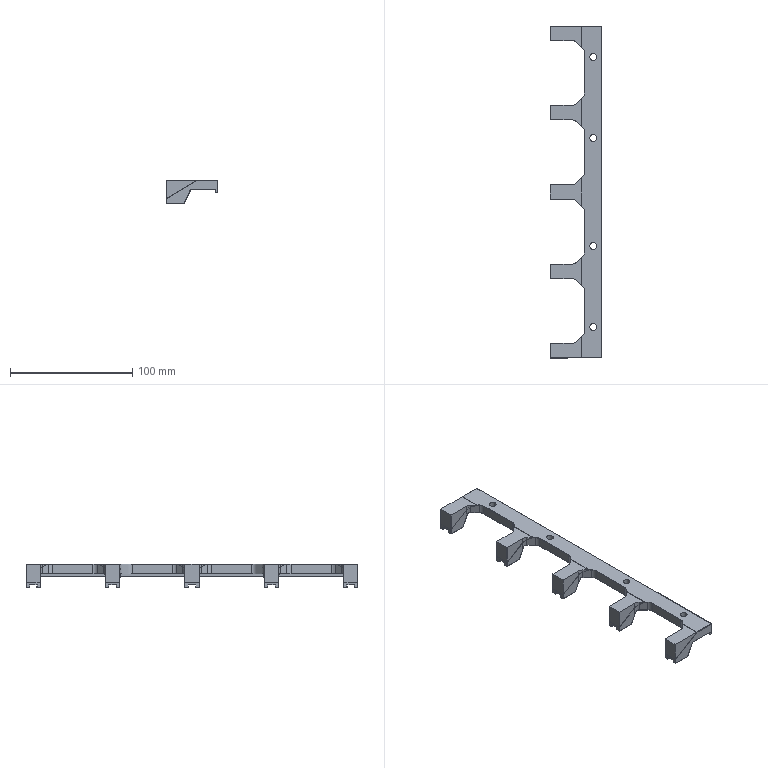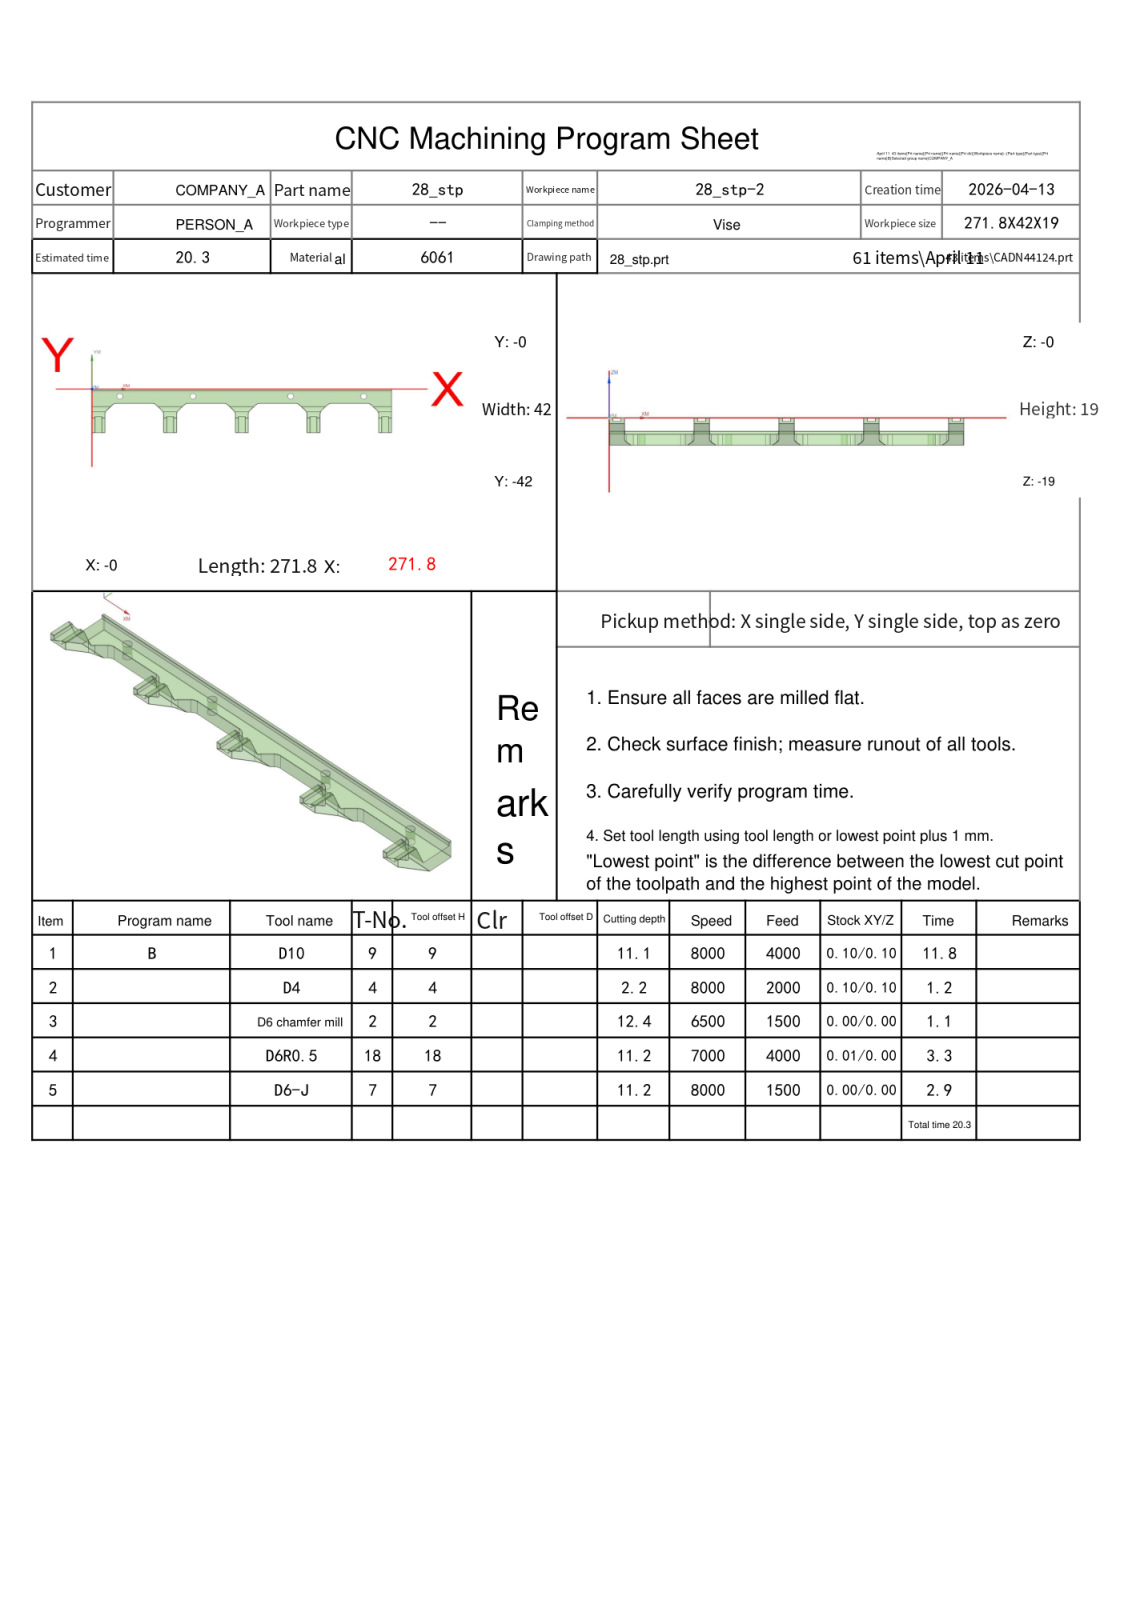NC program | NX | posted by the shop | part box 42 x 271.8 x 19 mm
Lines 6499 to 7627 of 14465:
N2 T04 M06
(D4  D=4. R=0. H=04 ce=0.10 di=0.10)
G00 G90 G54 X5.9 Y-47. M03 S8000
G43 H04 Z15.8
M08
Z1.225
G01 Z-.275 F2000.
Y-43.96
X3.71
X5. Y-42.67
Y-25.946
X3.72 Y-24.515
X8.08
X6.8 Y-25.946
Y-42.67
X8.09 Y-43.96
X5.9
X5.4
Y-47.
Z1.225
G00 X5.9
Z.95
G01 Z-.55
Y-43.96
X3.71
X5. Y-42.67
Y-25.946
X3.72 Y-24.515
X8.08
X6.8 Y-25.946
Y-42.67
X8.09 Y-43.96
X5.9
X5.4
Y-47.
Z.95
G00 X5.9
Z.675
G01 Z-.825
Y-43.96
X3.71
X5. Y-42.67
Y-25.946
X3.72 Y-24.515
X8.08
X6.8 Y-25.946
Y-42.67
X8.09 Y-43.96
X5.9
X5.4
Y-47.
Z.675
G00 X5.9
Z.4
G01 Z-1.1
Y-43.96
X3.71
X5. Y-42.67
Y-25.946
X3.72 Y-24.515
X8.08
X6.8 Y-25.946
Y-42.67
X8.09 Y-43.96
X5.9
X5.4
Y-47.
Z.4
G00 X5.9
Z.125
G01 Z-1.375
Y-43.96
X3.71
X5. Y-42.67
Y-25.946
X3.72 Y-24.515
X8.08
X6.8 Y-25.946
Y-42.67
X8.09 Y-43.96
X5.9
X5.4
Y-47.
Z.125
G00 X5.9
Z-.15
G01 Z-1.65
Y-43.96
X3.71
X5. Y-42.67
Y-25.946
X3.72 Y-24.515
X8.08
X6.8 Y-25.946
Y-42.67
X8.09 Y-43.96
X5.9
X5.4
Y-47.
Z-.15
G00 X5.9
Z-.425
G01 Z-1.925
Y-43.96
X3.71
X5. Y-42.67
Y-25.946
X3.72 Y-24.515
X8.08
X6.8 Y-25.946
Y-42.67
X8.09 Y-43.96
X5.9
X5.4
Y-47.
Z-.425
G00 X5.9
Z-.7
G01 Z-2.2
Y-43.96
X3.71
X5. Y-42.67
Y-25.946
X3.72 Y-24.515
X8.08
X6.8 Y-25.946
Y-42.67
X8.09 Y-43.96
X5.9
X5.4
Y-47.
Z-.7
G00 Z3.
X70.9
Z1.225
G01 Z-.275
Y-43.96
X68.71
X70. Y-42.67
Y-25.946
X68.72 Y-24.515
X73.08
X71.8 Y-25.946
Y-42.67
X73.09 Y-43.96
X70.9
X70.4
Y-47.
Z1.225
G00 X70.9
Z.95
G01 Z-.55
Y-43.96
X68.71
X70. Y-42.67
Y-25.946
X68.72 Y-24.515
X73.08
X71.8 Y-25.946
Y-42.67
X73.09 Y-43.96
X70.9
X70.4
Y-47.
Z.95
G00 X70.9
Z.675
G01 Z-.825
Y-43.96
X68.71
X70. Y-42.67
Y-25.946
X68.72 Y-24.515
X73.08
X71.8 Y-25.946
Y-42.67
X73.09 Y-43.96
X70.9
X70.4
Y-47.
Z.675
G00 X70.9
Z.4
G01 Z-1.1
Y-43.96
X68.71
X70. Y-42.67
Y-25.946
X68.72 Y-24.515
X73.08
X71.8 Y-25.946
Y-42.67
X73.09 Y-43.96
X70.9
X70.4
Y-47.
Z.4
G00 X70.9
Z.125
G01 Z-1.375
Y-43.96
X68.71
X70. Y-42.67
Y-25.946
X68.72 Y-24.515
X73.08
X71.8 Y-25.946
Y-42.67
X73.09 Y-43.96
X70.9
X70.4
Y-47.
Z.125
G00 X70.9
Z-.15
G01 Z-1.65
Y-43.96
X68.71
X70. Y-42.67
Y-25.946
X68.72 Y-24.515
X73.08
X71.8 Y-25.946
Y-42.67
X73.09 Y-43.96
X70.9
X70.4
Y-47.
Z-.15
G00 X70.9
Z-.425
G01 Z-1.925
Y-43.96
X68.71
X70. Y-42.67
Y-25.946
X68.72 Y-24.515
X73.08
X71.8 Y-25.946
Y-42.67
X73.09 Y-43.96
X70.9
X70.4
Y-47.
Z-.425
G00 X70.9
Z-.7
G01 Z-2.2
Y-43.96
X68.71
X70. Y-42.67
Y-25.946
X68.72 Y-24.515
X73.08
X71.8 Y-25.946
Y-42.67
X73.09 Y-43.96
X70.9
X70.4
Y-47.
Z-.7
G00 Z3.
X135.9
Z1.225
G01 Z-.275
Y-43.96
X133.71
X135. Y-42.67
Y-25.946
X133.72 Y-24.515
X138.08
X136.8 Y-25.946
Y-42.67
X138.09 Y-43.96
X135.9
X135.4
Y-47.
Z1.225
G00 X135.9
Z.95
G01 Z-.55
Y-43.96
X133.71
X135. Y-42.67
Y-25.946
X133.72 Y-24.515
X138.08
X136.8 Y-25.946
Y-42.67
X138.09 Y-43.96
X135.9
X135.4
Y-47.
Z.95
G00 X135.9
Z.675
G01 Z-.825
Y-43.96
X133.71
X135. Y-42.67
Y-25.946
X133.72 Y-24.515
X138.08
X136.8 Y-25.946
Y-42.67
X138.09 Y-43.96
X135.9
X135.4
Y-47.
Z.675
G00 X135.9
Z.4
G01 Z-1.1
Y-43.96
X133.71
X135. Y-42.67
Y-25.946
X133.72 Y-24.515
X138.08
X136.8 Y-25.946
Y-42.67
X138.09 Y-43.96
X135.9
X135.4
Y-47.
Z.4
G00 X135.9
Z.125
G01 Z-1.375
Y-43.96
X133.71
X135. Y-42.67
Y-25.946
X133.72 Y-24.515
X138.08
X136.8 Y-25.946
Y-42.67
X138.09 Y-43.96
X135.9
X135.4
Y-47.
Z.125
G00 X135.9
Z-.15
G01 Z-1.65
Y-43.96
X133.71
X135. Y-42.67
Y-25.946
X133.72 Y-24.515
X138.08
X136.8 Y-25.946
Y-42.67
X138.09 Y-43.96
X135.9
X135.4
Y-47.
Z-.15
G00 X135.9
Z-.425
G01 Z-1.925
Y-43.96
X133.71
X135. Y-42.67
Y-25.946
X133.72 Y-24.515
X138.08
X136.8 Y-25.946
Y-42.67
X138.09 Y-43.96
X135.9
X135.4
Y-47.
Z-.425
G00 X135.9
Z-.7
G01 Z-2.2
Y-43.96
X133.71
X135. Y-42.67
Y-25.946
X133.72 Y-24.515
X138.08
X136.8 Y-25.946
Y-42.67
X138.09 Y-43.96
X135.9
X135.4
Y-47.
Z-.7
G00 Z3.
X200.9
Z1.225
G01 Z-.275
Y-43.96
X198.71
X200. Y-42.67
Y-25.946
X198.72 Y-24.515
X203.08
X201.8 Y-25.946
Y-42.67
X203.09 Y-43.96
X200.9
X200.4
Y-47.
Z1.225
G00 X200.9
Z.95
G01 Z-.55
Y-43.96
X198.71
X200. Y-42.67
Y-25.946
X198.72 Y-24.515
X203.08
X201.8 Y-25.946
Y-42.67
X203.09 Y-43.96
X200.9
X200.4
Y-47.
Z.95
G00 X200.9
Z.675
G01 Z-.825
Y-43.96
X198.71
X200. Y-42.67
Y-25.946
X198.72 Y-24.515
X203.08
X201.8 Y-25.946
Y-42.67
X203.09 Y-43.96
X200.9
X200.4
Y-47.
Z.675
G00 X200.9
Z.4
G01 Z-1.1
Y-43.96
X198.71
X200. Y-42.67
Y-25.946
X198.72 Y-24.515
X203.08
X201.8 Y-25.946
Y-42.67
X203.09 Y-43.96
X200.9
X200.4
Y-47.
Z.4
G00 X200.9
Z.125
G01 Z-1.375
Y-43.96
X198.71
X200. Y-42.67
Y-25.946
X198.72 Y-24.515
X203.08
X201.8 Y-25.946
Y-42.67
X203.09 Y-43.96
X200.9
X200.4
Y-47.
Z.125
G00 X200.9
Z-.15
G01 Z-1.65
Y-43.96
X198.71
X200. Y-42.67
Y-25.946
X198.72 Y-24.515
X203.08
X201.8 Y-25.946
Y-42.67
X203.09 Y-43.96
X200.9
X200.4
Y-47.
Z-.15
G00 X200.9
Z-.425
G01 Z-1.925
Y-43.96
X198.71
X200. Y-42.67
Y-25.946
X198.72 Y-24.515
X203.08
X201.8 Y-25.946
Y-42.67
X203.09 Y-43.96
X200.9
X200.4
Y-47.
Z-.425
G00 X200.9
Z-.7
G01 Z-2.2
Y-43.96
X198.71
X200. Y-42.67
Y-25.946
X198.72 Y-24.515
X203.08
X201.8 Y-25.946
Y-42.67
X203.09 Y-43.96
X200.9
X200.4
Y-47.
Z-.7
G00 Z3.
X265.9
Z1.225
G01 Z-.275
Y-43.96
X263.71
X265. Y-42.67
Y-25.946
X263.72 Y-24.515
X268.08
X266.8 Y-25.946
Y-42.67
X268.09 Y-43.96
X265.9
X265.4
Y-47.
Z1.225
G00 X265.9
Z.95
G01 Z-.55
Y-43.96
X263.71
X265. Y-42.67
Y-25.946
X263.72 Y-24.515
X268.08
X266.8 Y-25.946
Y-42.67
X268.09 Y-43.96
X265.9
X265.4
Y-47.
Z.95
G00 X265.9
Z.675
G01 Z-.825
Y-43.96
X263.71
X265. Y-42.67
Y-25.946
X263.72 Y-24.515
X268.08
X266.8 Y-25.946
Y-42.67
X268.09 Y-43.96
X265.9
X265.4
Y-47.
Z.675
G00 X265.9
Z.4
G01 Z-1.1
Y-43.96
X263.71
X265. Y-42.67
Y-25.946
X263.72 Y-24.515
X268.08
X266.8 Y-25.946
Y-42.67
X268.09 Y-43.96
X265.9
X265.4
Y-47.
Z.4
G00 X265.9
Z.125
G01 Z-1.375
Y-43.96
X263.71
X265. Y-42.67
Y-25.946
X263.72 Y-24.515
X268.08
X266.8 Y-25.946
Y-42.67
X268.09 Y-43.96
X265.9
X265.4
Y-47.
Z.125
G00 X265.9
Z-.15
G01 Z-1.65
Y-43.96
X263.71
X265. Y-42.67
Y-25.946
X263.72 Y-24.515
X268.08
X266.8 Y-25.946
Y-42.67
X268.09 Y-43.96
X265.9
X265.4
Y-47.
Z-.15
G00 X265.9
Z-.425
G01 Z-1.925
Y-43.96
X263.71
X265. Y-42.67
Y-25.946
X263.72 Y-24.515
X268.08
X266.8 Y-25.946
Y-42.67
X268.09 Y-43.96
X265.9
X265.4
Y-47.
Z-.425
G00 X265.9
Z-.7
G01 Z-2.2
Y-43.96
X263.71
X265. Y-42.67
Y-25.946
X263.72 Y-24.515
X268.08
X266.8 Y-25.946
Y-42.67
X268.09 Y-43.96
X265.9
X265.4
Y-47.
Z-.7
G00 Z15.8
G91 G28 Z0.0
M05
M09
G91 G28 Z0.0
M01
N3 T02 M06
(D6 chamfer mill  D=6. R=0. H=02 ce=0.00 di=0.00)
G00 G90 G54 X272.615 Y-27.282 M03 S6500
G43 H02 Z20.
M08
Z2.8
G01 Z-1.2 F1500.
X272.684 Y-27.381
X272.771 Y-27.608
X272.8 Y-27.849
Y-41.8
X272.766 Y-42.059
X272.666 Y-42.3
X272.507 Y-42.507
X272.307 Y-42.707
X272.1 Y-42.866
X271.859 Y-42.966
X271.6 Y-43.
X269.1
X268.841 Y-42.966
X268.6 Y-42.866
X268.393 Y-42.707
X268.193 Y-42.507
X268.034 Y-42.3
X267.934 Y-42.059
X267.9 Y-41.8
Y-34.824
Y-27.849
X267.929 Y-27.608
X268.016 Y-27.381
X268.085 Y-27.282
Z2.8
G00 X263.715
G01 Z-1.2
X263.784 Y-27.381
X263.871 Y-27.608
X263.9 Y-27.849
Y-34.824
Y-41.8
X263.866 Y-42.059
X263.766 Y-42.3
X263.607 Y-42.507
X263.407 Y-42.707
X263.2 Y-42.866
X262.959 Y-42.966
X262.7 Y-43.
X260.1
X259.841 Y-42.966
X259.6 Y-42.866
X259.393 Y-42.707
X259.193 Y-42.507
X259.034 Y-42.3
X258.934 Y-42.059
X258.9 Y-41.8
Y-27.849
X258.929 Y-27.608
X259.016 Y-27.381
X259.085 Y-27.282
Z2.8
G00 Z10.
X207.715
Z2.8
G01 Z-1.2
X207.784 Y-27.381
X207.871 Y-27.608
X207.9 Y-27.849
Y-34.824
Y-41.8
X207.866 Y-42.059
X207.766 Y-42.3
X207.607 Y-42.507
X207.407 Y-42.707
X207.2 Y-42.866
X206.959 Y-42.966
X206.7 Y-43.
X204.1
X203.841 Y-42.966
X203.6 Y-42.866
X203.393 Y-42.707
X203.193 Y-42.507
X203.034 Y-42.3
X202.934 Y-42.059
X202.9 Y-41.8
Y-27.849
X202.929 Y-27.608
X203.016 Y-27.381
X203.085 Y-27.282
Z2.8
G00 X198.715
G01 Z-1.2
X198.784 Y-27.381
X198.871 Y-27.608
X198.9 Y-27.849
Y-34.824
Y-41.8
X198.866 Y-42.059
X198.766 Y-42.3
X198.607 Y-42.507
X198.407 Y-42.707
X198.2 Y-42.866
X197.959 Y-42.966
X197.7 Y-43.
X195.1
X194.841 Y-42.966
X194.6 Y-42.866
X194.393 Y-42.707
X194.193 Y-42.507
X194.034 Y-42.3
X193.934 Y-42.059
X193.9 Y-41.8
Y-27.849
X193.929 Y-27.608
X194.016 Y-27.381
X194.085 Y-27.282
Z2.8
G00 Z10.
X142.715
Z2.8
G01 Z-1.2
X142.784 Y-27.381
X142.871 Y-27.608
X142.9 Y-27.849
Y-34.824
Y-41.8
X142.866 Y-42.059
X142.766 Y-42.3
X142.607 Y-42.507
X142.407 Y-42.707
X142.2 Y-42.866
X141.959 Y-42.966
X141.7 Y-43.
X139.1
X138.841 Y-42.966
X138.6 Y-42.866
X138.393 Y-42.707
X138.193 Y-42.507
X138.034 Y-42.3
X137.934 Y-42.059
X137.9 Y-41.8
Y-27.849
X137.929 Y-27.608
X138.016 Y-27.381
X138.085 Y-27.282
Z2.8
G00 X133.715
G01 Z-1.2
X133.784 Y-27.381
X133.871 Y-27.608
X133.9 Y-27.849
Y-34.824
Y-41.8
X133.866 Y-42.059
X133.766 Y-42.3
X133.607 Y-42.507
X133.407 Y-42.707
X133.2 Y-42.866
X132.959 Y-42.966
X132.7 Y-43.
X130.1
X129.841 Y-42.966
X129.6 Y-42.866
X129.393 Y-42.707
X129.193 Y-42.507
X129.034 Y-42.3
X128.934 Y-42.059
X128.9 Y-41.8
Y-27.849
X128.929 Y-27.608
X129.016 Y-27.381
X129.085 Y-27.282
Z2.8
G00 Z10.
X77.715
Z2.8
G01 Z-1.2
X77.784 Y-27.381
X77.871 Y-27.608
X77.9 Y-27.849
Y-41.8
X77.866 Y-42.059
X77.766 Y-42.3
X77.607 Y-42.507
X77.407 Y-42.707
X77.2 Y-42.866
X76.959 Y-42.966
X76.7 Y-43.
X74.1
X73.841 Y-42.966
X73.6 Y-42.866
X73.393 Y-42.707
X73.193 Y-42.507
X73.034 Y-42.3
X72.934 Y-42.059
X72.9 Y-41.8
Y-34.824
Y-27.849
X72.929 Y-27.608
X73.016 Y-27.381
X73.085 Y-27.282
Z2.8
G00 X68.715
G01 Z-1.2
X68.784 Y-27.381
X68.871 Y-27.608
X68.9 Y-27.849
Y-41.8
X68.866 Y-42.059
X68.766 Y-42.3
X68.607 Y-42.507
X68.407 Y-42.707
X68.2 Y-42.866
X67.959 Y-42.966
X67.7 Y-43.
X65.1
X64.841 Y-42.966
X64.6 Y-42.866
X64.393 Y-42.707
X64.193 Y-42.507
X64.034 Y-42.3
X63.934 Y-42.059
X63.9 Y-41.8
Y-34.824
Y-27.849
X63.929 Y-27.608
X64.016 Y-27.381
X64.085 Y-27.282
Z2.8
G00 Z10.
X12.715
Z2.8
G01 Z-1.2
X12.784 Y-27.381
X12.871 Y-27.608
X12.9 Y-27.849
Y-34.824
Y-41.8
X12.866 Y-42.059
X12.766 Y-42.3
X12.607 Y-42.507
X12.407 Y-42.707
X12.2 Y-42.866
X11.959 Y-42.966
X11.7 Y-43.
X9.1
X8.841 Y-42.966
X8.6 Y-42.866
X8.393 Y-42.707
X8.193 Y-42.507
X8.034 Y-42.3
X7.934 Y-42.059
X7.9 Y-41.8
Y-27.849
X7.929 Y-27.608
X8.016 Y-27.381
X8.085 Y-27.282
Z2.8
G00 X3.715
G01 Z-1.2
X3.784 Y-27.381
X3.871 Y-27.608
X3.9 Y-27.849
Y-34.824
Y-41.8
X3.866 Y-42.059
X3.766 Y-42.3
X3.607 Y-42.507
X3.407 Y-42.707
X3.2 Y-42.866
X2.959 Y-42.966
X2.7 Y-43.
X.2
X-.059 Y-42.966
X-.3 Y-42.866
X-.507 Y-42.707
X-.707 Y-42.507
X-.866 Y-42.3
X-.966 Y-42.059
X-1. Y-41.8
Y-27.849
X-.971 Y-27.608
X-.884 Y-27.381
X-.815 Y-27.282
Z2.8
G00 Z10.
X136.286 Y-3.177
Z-9.078
G01 Z-10.45
G03 X136. Y-2.977 I-1.286 J-1.532
G01 X135.954 Y-2.947
X135.9 Y-2.95
X.1
X-.159 Y-2.916
X-.4 Y-2.816
X-.607 Y-2.657
X-.707 Y-2.557
X-.866 Y-2.35
X-.966 Y-2.109
X-1. Y-1.85
Y-.5
X-.966 Y-.241
X-.866 Y0.0
X-.707 Y.207
X-.207 Y.707
X0.0 Y.866
X.241 Y.966
X.5 Y1.
X271.3
X271.559 Y.966
X271.8 Y.866
X272.007 Y.707
X272.507 Y.207
X272.666 Y0.0
X272.766 Y-.241
X272.8 Y-.5
Y-1.85
X272.766 Y-2.109
X272.666 Y-2.35
X272.507 Y-2.557
X272.407 Y-2.657
X272.2 Y-2.816
X271.959 Y-2.916
X271.7 Y-2.95
X135.9
X135.846 Y-2.947
X135.8 Y-2.977
G03 X135.514 Y-3.177 I1. J-1.732
G01 Z-9.078
G00 Z10.
X192.493 Y-21.072
Z-8.673
G01 Z-12.45
X192.481 Y-21.003
X192.471 Y-20.985
X187.657 Y-16.172
G03 X184.829 Y-15. I-2.828 J-2.828
G01 X151.971
G03 X149.143 Y-16.172 I0.0 J-4.
G01 X144.329 Y-20.985
X144.319 Y-21.003
X144.307 Y-21.072
Z-8.673
G00 Z10.
X257.533 Y-21.111
Z-8.534
G01 Z-12.45
X257.521 Y-21.043
X257.511 Y-21.025
X252.657 Y-16.172
G03 X249.829 Y-15. I-2.828 J-2.828
G01 X216.971
G03 X214.143 Y-16.172 I0.0 J-4.
G01 X209.329 Y-20.985
X209.319 Y-21.003
X209.307 Y-21.072
Z-8.673
G00 Z10.
X272.891 Y-4.879
Z-10.942
G01 Z-12.45
X272.84 Y-4.929
X272.811 Y-4.993
X272.793 Y-5.01
X272.8 Y-5.033
Y-19.955
X272.793 Y-19.979
X272.811 Y-19.995
X272.84 Y-20.06
X272.891 Y-20.11
Z-9.187
G00 Z10.
X-1.091
Z-9.187
G01 Z-12.45
X-1.04 Y-20.06
X-1.011 Y-19.995
X-.993 Y-19.979
X-1. Y-19.955
Y-5.004
X-1.008 Y-4.974
X-1.068 Y-4.888
Z-10.919
G00 Z10.
X62.493 Y-21.072
Z-8.673
G01 Z-12.45
X62.481 Y-21.003
X62.471 Y-20.985
X57.657 Y-16.172
G03 X54.829 Y-15. I-2.828 J-2.828
G01 X21.971
G03 X19.143 Y-16.172 I0.0 J-4.
G01 X14.329 Y-20.985
X14.319 Y-21.003
X14.307 Y-21.072
Z-8.673
G00 Z10.
X127.493
Z-8.673
G01 Z-12.45
X127.481 Y-21.003
X127.471 Y-20.985
X122.657 Y-16.172
G03 X119.829 Y-15. I-2.828 J-2.828
G01 X86.971
G03 X84.143 Y-16.172 I0.0 J-4.
G01 X79.329 Y-20.985
X79.319 Y-21.003
X79.307 Y-21.072
Z-8.673
G00 Z10.
X25.707 Y-5.435
Z-10.975
G01 Z-12.45
G03 X25.402 Y-5.266 I-1.118 J-1.658
G01 X25.354 Y-5.241
X25.3 Y-5.25
G03 X23.55 Y-7. I0.0 J-1.75
X25.3 Y-8.75 I1.75 J0.0
X27.05 Y-7. I0.0 J1.75
X25.3 Y-5.25 I-1.75 J0.0
G01 X25.246 Y-5.241
X25.198 Y-5.266
G03 X24.893 Y-5.435 I.813 J-1.827
G01 Z-10.975
G00 Z10.
X92.007
Z-10.975
G01 Z-12.45
G03 X91.702 Y-5.266 I-1.118 J-1.658
G01 X91.654 Y-5.241
X91.6 Y-5.25
G03 X89.85 Y-7. I0.0 J-1.75
X91.6 Y-8.75 I1.75 J0.0
X93.35 Y-7. I0.0 J1.75
X91.6 Y-5.25 I-1.75 J0.0
G01 X91.546 Y-5.241
X91.498 Y-5.266
G03 X91.193 Y-5.435 I.813 J-1.827
G01 Z-10.975
G00 Z10.
X180.607
Z-10.975
G01 Z-12.45
G03 X180.302 Y-5.266 I-1.118 J-1.658
G01 X180.254 Y-5.241
X180.2 Y-5.25
G03 X178.45 Y-7. I0.0 J-1.75
X180.2 Y-8.75 I1.75 J0.0
X181.95 Y-7. I0.0 J1.75
X180.2 Y-5.25 I-1.75 J0.0
G01 X180.146 Y-5.241
X180.098 Y-5.266
G03 X179.793 Y-5.435 I.813 J-1.827
G01 Z-10.975
G00 Z10.
X246.907
Z-10.975
G01 Z-12.45
G03 X246.602 Y-5.266 I-1.118 J-1.658
G01 X246.554 Y-5.241
X246.5 Y-5.25
G03 X244.75 Y-7. I0.0 J-1.75
X246.5 Y-8.75 I1.75 J0.0
X248.25 Y-7. I0.0 J1.75
X246.5 Y-5.25 I-1.75 J0.0
G01 X246.446 Y-5.241
X246.398 Y-5.266
G03 X246.093 Y-5.435 I.813 J-1.827
G01 Z-10.975
G00 Z20.
G91 G28 Z0.0
M05
M09
G91 G28 Z0.0
M01